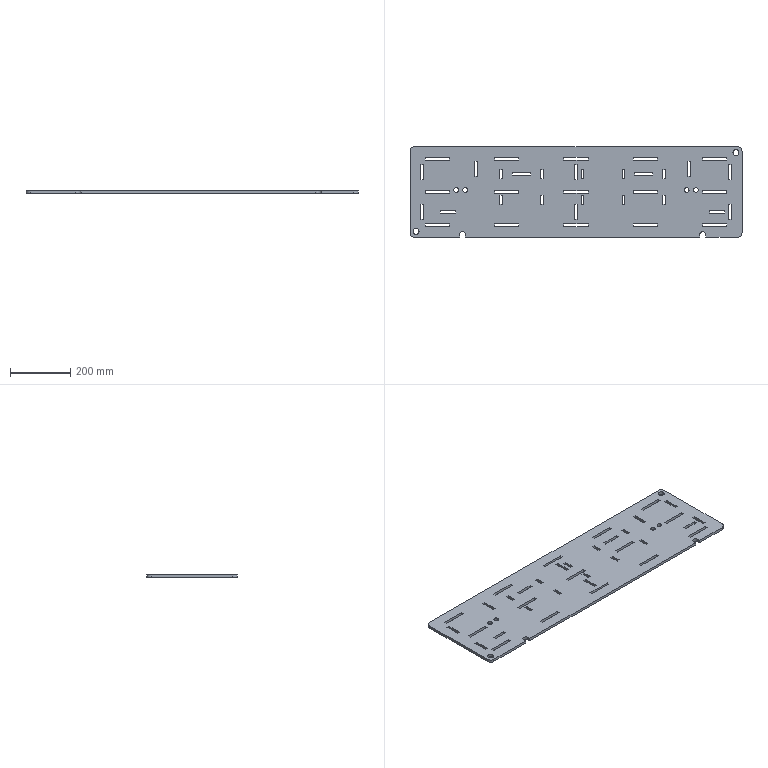Part | SolidWorks | features FlatPattern 1, SMBaseFlange 1, SheetMetal 1 | 1 solid | 178 faces | box 1100 x 300 x 9 mm | volume 2778509 mm3 | plane 160 | cylinder 18 | commonest cylinder face diameters 15 x4 15.5 x4 20 x4 30 x4 19 x2